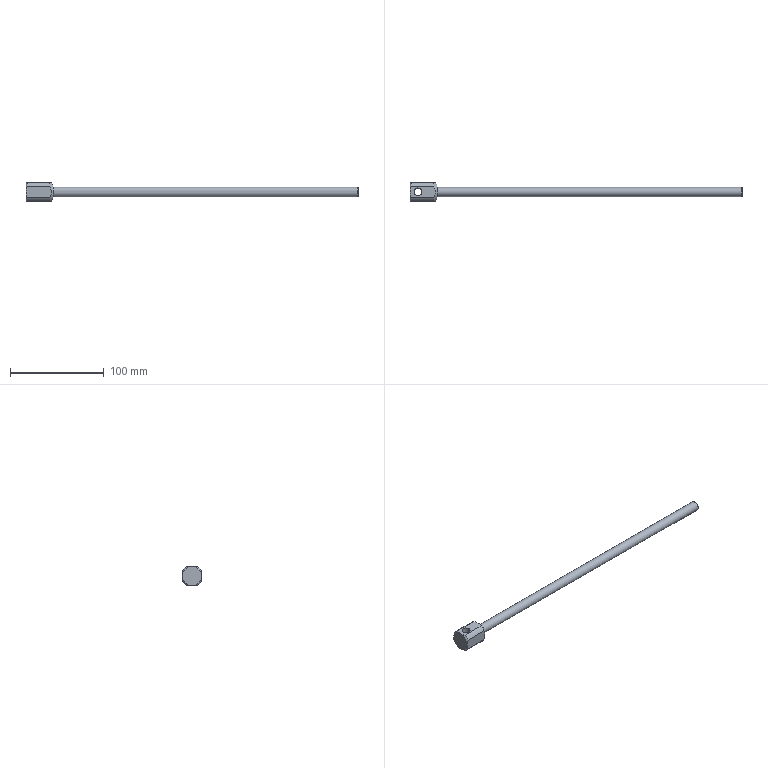Part | STEP file | GAS SHOCK 608S | 1 solid | 20 faces | box 353.5 x 20 x 20 mm | volume 34694 mm3 | plane 7 | cylinder 6 | cone 5 | torus 2 | commonest cylinder face diameters 23 x4 8.5 x1 10 x1
STEP:
#1=CARTESIAN_POINT('',(-27.,-10.,-5.679));
#2=VERTEX_POINT('',#1);
#3=CARTESIAN_POINT('',(-27.,-5.679,-10.));
#4=VERTEX_POINT('',#3);
#5=CARTESIAN_POINT('',(-27.,0.,0.));
#6=DIRECTION('',(1.,0.,0.));
#7=DIRECTION('',(0.,0.,1.));
#8=AXIS2_PLACEMENT_3D('',#5,#6,#7);
#9=CIRCLE('',#8,11.5);
#10=EDGE_CURVE('',#2,#4,#9,.T.);
#11=ORIENTED_EDGE('',*,*,#10,.T.);
#12=CARTESIAN_POINT('',(-3.,-5.679,-10.));
#13=VERTEX_POINT('',#12);
#14=CARTESIAN_POINT('',(-28.5,-5.679,-10.));
#15=DIRECTION('',(1.,0.,0.));
#16=VECTOR('',#15,1000.);
#17=LINE('',#14,#16);
#18=EDGE_CURVE('',#4,#13,#17,.T.);
#19=ORIENTED_EDGE('',*,*,#18,.T.);
#20=CARTESIAN_POINT('',(-3.,-10.,-5.679));
#21=VERTEX_POINT('',#20);
#22=CARTESIAN_POINT('',(-3.,0.,0.));
#23=DIRECTION('',(-1.,0.,0.));
#24=DIRECTION('',(0.,0.,1.));
#25=AXIS2_PLACEMENT_3D('',#22,#23,#24);
#26=CIRCLE('',#25,11.5);
#27=EDGE_CURVE('',#13,#21,#26,.T.);
#28=ORIENTED_EDGE('',*,*,#27,.T.);
#29=CARTESIAN_POINT('',(-28.5,-10.,-5.679));
#30=DIRECTION('',(-1.,0.,0.));
#31=VECTOR('',#30,1000.);
#32=LINE('',#29,#31);
#33=EDGE_CURVE('',#21,#2,#32,.T.);
#34=ORIENTED_EDGE('',*,*,#33,.T.);
#35=EDGE_LOOP('',(#11,#19,#28,#34));
#36=FACE_OUTER_BOUND('',#35,.T.);
#37=CARTESIAN_POINT('',(-28.5,0.,0.));
#38=DIRECTION('',(1.,0.,0.));
#39=DIRECTION('',(0.,0.,-1.));
#40=AXIS2_PLACEMENT_3D('',#37,#38,#39);
#41=CYLINDRICAL_SURFACE('',#40,11.5);
#42=ADVANCED_FACE('',(#36),#41,.T.);
#43=CARTESIAN_POINT('',(-28.5,0.,-10.));
#44=VERTEX_POINT('',#43);
#45=CARTESIAN_POINT('',(-27.,-5.679,-10.));
#46=CARTESIAN_POINT('',(-27.44,-4.788,-10.));
#47=CARTESIAN_POINT('',(-27.813,-3.877,-10.));
#48=CARTESIAN_POINT('',(-28.211,-2.462,-10.));
#49=CARTESIAN_POINT('',(-28.317,-1.982,-10.));
#50=CARTESIAN_POINT('',(-28.462,-1.001,-10.));
#51=CARTESIAN_POINT('',(-28.5,-0.4969,-10.));
#52=CARTESIAN_POINT('',(-28.5,0.,-10.));
#53=B_SPLINE_CURVE_WITH_KNOTS('',3,(#45,#46,#47,#48,#49,#50,#51,#52),.UNSPECIFIED.,.F.,.F.,(4,2,2,4),(0.01277,0.01572,0.01719,0.01867),.UNSPECIFIED.);
#54=EDGE_CURVE('',#4,#44,#53,.T.);
#55=ORIENTED_EDGE('',*,*,#54,.F.);
#56=ORIENTED_EDGE('',*,*,#10,.F.);
#57=CARTESIAN_POINT('',(-28.5,-10.,0.));
#58=VERTEX_POINT('',#57);
#59=CARTESIAN_POINT('',(-28.5,-10.,0.));
#60=CARTESIAN_POINT('',(-28.5,-10.,-0.2479));
#61=CARTESIAN_POINT('',(-28.491,-10.,-0.4984));
#62=CARTESIAN_POINT('',(-28.454,-10.,-0.996));
#63=CARTESIAN_POINT('',(-28.426,-10.,-1.242));
#64=CARTESIAN_POINT('',(-28.318,-10.,-1.975));
#65=CARTESIAN_POINT('',(-28.213,-10.,-2.454));
#66=CARTESIAN_POINT('',(-27.948,-10.,-3.398));
#67=CARTESIAN_POINT('',(-27.788,-10.,-3.863));
#68=CARTESIAN_POINT('',(-27.424,-10.,-4.781));
#69=CARTESIAN_POINT('',(-27.219,-10.,-5.235));
#70=CARTESIAN_POINT('',(-27.,-10.,-5.679));
#71=B_SPLINE_CURVE_WITH_KNOTS('',3,(#59,#60,#61,#62,#63,#64,#65,#66,#67,#68,#69,#70),.UNSPECIFIED.,.F.,.F.,(4,2,2,2,2,4),(0.01208,0.01282,0.01355,0.01502,0.01649,0.01796),.UNSPECIFIED.);
#72=EDGE_CURVE('',#58,#2,#71,.T.);
#73=ORIENTED_EDGE('',*,*,#72,.F.);
#74=CARTESIAN_POINT('',(-28.5,0.,0.));
#75=DIRECTION('',(-1.,0.,0.));
#76=DIRECTION('',(0.,0.,1.));
#77=AXIS2_PLACEMENT_3D('',#74,#75,#76);
#78=CIRCLE('',#77,10.);
#79=EDGE_CURVE('',#44,#58,#78,.T.);
#80=ORIENTED_EDGE('',*,*,#79,.F.);
#81=EDGE_LOOP('',(#55,#56,#73,#80));
#82=FACE_OUTER_BOUND('',#81,.T.);
#83=CARTESIAN_POINT('',(-28.5,0.,0.));
#84=DIRECTION('',(1.,0.,0.));
#85=DIRECTION('',(0.,0.,-1.));
#86=AXIS2_PLACEMENT_3D('',#83,#84,#85);
#87=CONICAL_SURFACE('',#86,10.,0.7854);
#88=ADVANCED_FACE('',(#82),#87,.T.);
#89=CARTESIAN_POINT('',(-27.,-5.679,10.));
#90=VERTEX_POINT('',#89);
#91=CARTESIAN_POINT('',(-27.,-10.,5.679));
#92=VERTEX_POINT('',#91);
#93=CARTESIAN_POINT('',(-27.,0.,0.));
#94=DIRECTION('',(1.,0.,0.));
#95=DIRECTION('',(0.,0.,1.));
#96=AXIS2_PLACEMENT_3D('',#93,#94,#95);
#97=CIRCLE('',#96,11.5);
#98=EDGE_CURVE('',#90,#92,#97,.T.);
#99=ORIENTED_EDGE('',*,*,#98,.T.);
#100=CARTESIAN_POINT('',(-3.,-10.,5.679));
#101=VERTEX_POINT('',#100);
#102=CARTESIAN_POINT('',(-28.5,-10.,5.679));
#103=DIRECTION('',(1.,0.,0.));
#104=VECTOR('',#103,1000.);
#105=LINE('',#102,#104);
#106=EDGE_CURVE('',#92,#101,#105,.T.);
#107=ORIENTED_EDGE('',*,*,#106,.T.);
#108=CARTESIAN_POINT('',(-3.,-5.679,10.));
#109=VERTEX_POINT('',#108);
#110=CARTESIAN_POINT('',(-3.,0.,0.));
#111=DIRECTION('',(-1.,0.,0.));
#112=DIRECTION('',(0.,0.,1.));
#113=AXIS2_PLACEMENT_3D('',#110,#111,#112);
#114=CIRCLE('',#113,11.5);
#115=EDGE_CURVE('',#101,#109,#114,.T.);
#116=ORIENTED_EDGE('',*,*,#115,.T.);
#117=CARTESIAN_POINT('',(-28.5,-5.679,10.));
#118=DIRECTION('',(-1.,0.,0.));
#119=VECTOR('',#118,1000.);
#120=LINE('',#117,#119);
#121=EDGE_CURVE('',#109,#90,#120,.T.);
#122=ORIENTED_EDGE('',*,*,#121,.T.);
#123=EDGE_LOOP('',(#99,#107,#116,#122));
#124=FACE_OUTER_BOUND('',#123,.T.);
#125=CARTESIAN_POINT('',(-28.5,0.,0.));
#126=DIRECTION('',(1.,0.,0.));
#127=DIRECTION('',(0.,0.,-1.));
#128=AXIS2_PLACEMENT_3D('',#125,#126,#127);
#129=CYLINDRICAL_SURFACE('',#128,11.5);
#130=ADVANCED_FACE('',(#124),#129,.T.);
#131=CARTESIAN_POINT('',(-27.,-10.,5.679));
#132=CARTESIAN_POINT('',(-27.218,-10.,5.238));
#133=CARTESIAN_POINT('',(-27.421,-10.,4.789));
#134=CARTESIAN_POINT('',(-27.787,-10.,3.867));
#135=CARTESIAN_POINT('',(-27.95,-10.,3.392));
#136=CARTESIAN_POINT('',(-28.35,-10.,1.964));
#137=CARTESIAN_POINT('',(-28.5,-10.,0.9934));
#138=CARTESIAN_POINT('',(-28.5,-10.,0.));
#139=B_SPLINE_CURVE_WITH_KNOTS('',3,(#131,#132,#133,#134,#135,#136,#137,#138),.UNSPECIFIED.,.F.,.F.,(4,2,2,4),(0.006195,0.007667,0.00914,0.01208),.UNSPECIFIED.);
#140=EDGE_CURVE('',#92,#58,#139,.T.);
#141=ORIENTED_EDGE('',*,*,#140,.F.);
#142=ORIENTED_EDGE('',*,*,#98,.F.);
#143=CARTESIAN_POINT('',(-28.5,0.,10.));
#144=VERTEX_POINT('',#143);
#145=CARTESIAN_POINT('',(-28.5,0.,10.));
#146=CARTESIAN_POINT('',(-28.5,-0.2479,10.));
#147=CARTESIAN_POINT('',(-28.491,-0.4984,10.));
#148=CARTESIAN_POINT('',(-28.454,-0.996,10.));
#149=CARTESIAN_POINT('',(-28.426,-1.242,10.));
#150=CARTESIAN_POINT('',(-28.318,-1.975,10.));
#151=CARTESIAN_POINT('',(-28.213,-2.454,10.));
#152=CARTESIAN_POINT('',(-27.948,-3.398,10.));
#153=CARTESIAN_POINT('',(-27.788,-3.863,10.));
#154=CARTESIAN_POINT('',(-27.424,-4.781,10.));
#155=CARTESIAN_POINT('',(-27.219,-5.235,10.));
#156=CARTESIAN_POINT('',(-27.,-5.679,10.));
#157=B_SPLINE_CURVE_WITH_KNOTS('',3,(#145,#146,#147,#148,#149,#150,#151,#152,#153,#154,#155,#156),.UNSPECIFIED.,.F.,.F.,(4,2,2,2,2,4),(0.01208,0.01282,0.01355,0.01502,0.01649,0.01796),.UNSPECIFIED.);
#158=EDGE_CURVE('',#144,#90,#157,.T.);
#159=ORIENTED_EDGE('',*,*,#158,.F.);
#160=CARTESIAN_POINT('',(-28.5,0.,0.));
#161=DIRECTION('',(-1.,0.,0.));
#162=DIRECTION('',(0.,0.,1.));
#163=AXIS2_PLACEMENT_3D('',#160,#161,#162);
#164=CIRCLE('',#163,10.);
#165=EDGE_CURVE('',#58,#144,#164,.T.);
#166=ORIENTED_EDGE('',*,*,#165,.F.);
#167=EDGE_LOOP('',(#141,#142,#159,#166));
#168=FACE_OUTER_BOUND('',#167,.T.);
#169=CARTESIAN_POINT('',(-28.5,0.,0.));
#170=DIRECTION('',(1.,0.,0.));
#171=DIRECTION('',(0.,0.,-1.));
#172=AXIS2_PLACEMENT_3D('',#169,#170,#171);
#173=CONICAL_SURFACE('',#172,10.,0.7854);
#174=ADVANCED_FACE('',(#168),#173,.T.);
#175=CARTESIAN_POINT('',(-27.,10.,5.679));
#176=VERTEX_POINT('',#175);
#177=CARTESIAN_POINT('',(-27.,5.679,10.));
#178=VERTEX_POINT('',#177);
#179=CARTESIAN_POINT('',(-27.,0.,0.));
#180=DIRECTION('',(1.,0.,0.));
#181=DIRECTION('',(0.,0.,1.));
#182=AXIS2_PLACEMENT_3D('',#179,#180,#181);
#183=CIRCLE('',#182,11.5);
#184=EDGE_CURVE('',#176,#178,#183,.T.);
#185=ORIENTED_EDGE('',*,*,#184,.T.);
#186=CARTESIAN_POINT('',(-3.,5.679,10.));
#187=VERTEX_POINT('',#186);
#188=CARTESIAN_POINT('',(-28.5,5.679,10.));
#189=DIRECTION('',(1.,0.,0.));
#190=VECTOR('',#189,1000.);
#191=LINE('',#188,#190);
#192=EDGE_CURVE('',#178,#187,#191,.T.);
#193=ORIENTED_EDGE('',*,*,#192,.T.);
#194=CARTESIAN_POINT('',(-3.,10.,5.679));
#195=VERTEX_POINT('',#194);
#196=CARTESIAN_POINT('',(-3.,0.,0.));
#197=DIRECTION('',(-1.,0.,0.));
#198=DIRECTION('',(0.,0.,1.));
#199=AXIS2_PLACEMENT_3D('',#196,#197,#198);
#200=CIRCLE('',#199,11.5);
#201=EDGE_CURVE('',#187,#195,#200,.T.);
#202=ORIENTED_EDGE('',*,*,#201,.T.);
#203=CARTESIAN_POINT('',(-28.5,10.,5.679));
#204=DIRECTION('',(-1.,0.,0.));
#205=VECTOR('',#204,1000.);
#206=LINE('',#203,#205);
#207=EDGE_CURVE('',#195,#176,#206,.T.);
#208=ORIENTED_EDGE('',*,*,#207,.T.);
#209=EDGE_LOOP('',(#185,#193,#202,#208));
#210=FACE_OUTER_BOUND('',#209,.T.);
#211=CARTESIAN_POINT('',(-28.5,0.,0.));
#212=DIRECTION('',(1.,0.,0.));
#213=DIRECTION('',(0.,0.,-1.));
#214=AXIS2_PLACEMENT_3D('',#211,#212,#213);
#215=CYLINDRICAL_SURFACE('',#214,11.5);
#216=ADVANCED_FACE('',(#210),#215,.T.);
#217=CARTESIAN_POINT('',(-27.,5.679,10.));
#218=CARTESIAN_POINT('',(-27.218,5.238,10.));
#219=CARTESIAN_POINT('',(-27.421,4.789,10.));
#220=CARTESIAN_POINT('',(-27.787,3.867,10.));
#221=CARTESIAN_POINT('',(-27.95,3.392,10.));
#222=CARTESIAN_POINT('',(-28.35,1.964,10.));
#223=CARTESIAN_POINT('',(-28.5,0.9934,10.));
#224=CARTESIAN_POINT('',(-28.5,0.,10.));
#225=B_SPLINE_CURVE_WITH_KNOTS('',3,(#217,#218,#219,#220,#221,#222,#223,#224),.UNSPECIFIED.,.F.,.F.,(4,2,2,4),(0.006195,0.007667,0.00914,0.01208),.UNSPECIFIED.);
#226=EDGE_CURVE('',#178,#144,#225,.T.);
#227=ORIENTED_EDGE('',*,*,#226,.F.);
#228=ORIENTED_EDGE('',*,*,#184,.F.);
#229=CARTESIAN_POINT('',(-28.5,10.,0.));
#230=VERTEX_POINT('',#229);
#231=CARTESIAN_POINT('',(-28.5,10.,0.));
#232=CARTESIAN_POINT('',(-28.5,10.,0.9898));
#233=CARTESIAN_POINT('',(-28.351,10.,1.963));
#234=CARTESIAN_POINT('',(-27.812,10.,3.883));
#235=CARTESIAN_POINT('',(-27.436,10.,4.796));
#236=CARTESIAN_POINT('',(-27.,10.,5.679));
#237=B_SPLINE_CURVE_WITH_KNOTS('',3,(#231,#232,#233,#234,#235,#236),.UNSPECIFIED.,.F.,.F.,(4,2,4),(0.01867,0.0216,0.02454),.UNSPECIFIED.);
#238=EDGE_CURVE('',#230,#176,#237,.T.);
#239=ORIENTED_EDGE('',*,*,#238,.F.);
#240=CARTESIAN_POINT('',(-28.5,0.,0.));
#241=DIRECTION('',(-1.,0.,0.));
#242=DIRECTION('',(0.,0.,1.));
#243=AXIS2_PLACEMENT_3D('',#240,#241,#242);
#244=CIRCLE('',#243,10.);
#245=EDGE_CURVE('',#144,#230,#244,.T.);
#246=ORIENTED_EDGE('',*,*,#245,.F.);
#247=EDGE_LOOP('',(#227,#228,#239,#246));
#248=FACE_OUTER_BOUND('',#247,.T.);
#249=CARTESIAN_POINT('',(-28.5,0.,0.));
#250=DIRECTION('',(1.,0.,0.));
#251=DIRECTION('',(0.,0.,-1.));
#252=AXIS2_PLACEMENT_3D('',#249,#250,#251);
#253=CONICAL_SURFACE('',#252,10.,0.7854);
#254=ADVANCED_FACE('',(#248),#253,.T.);
#255=CARTESIAN_POINT('',(0.5,0.,5.));
#256=VERTEX_POINT('',#255);
#257=CARTESIAN_POINT('',(0.5,0.,0.));
#258=DIRECTION('',(1.,0.,0.));
#259=DIRECTION('',(0.,0.,1.));
#260=AXIS2_PLACEMENT_3D('',#257,#258,#259);
#261=CIRCLE('',#260,5.);
#262=EDGE_CURVE('',#256,#256,#261,.T.);
#263=ORIENTED_EDGE('',*,*,#262,.T.);
#264=EDGE_LOOP('',(#263));
#265=FACE_OUTER_BOUND('',#264,.T.);
#266=CARTESIAN_POINT('',(324.5,0.,-5.));
#267=VERTEX_POINT('',#266);
#268=CARTESIAN_POINT('',(324.5,0.,0.));
#269=DIRECTION('',(-1.,0.,0.));
#270=DIRECTION('',(0.,0.,-1.));
#271=AXIS2_PLACEMENT_3D('',#268,#269,#270);
#272=CIRCLE('',#271,5.);
#273=EDGE_CURVE('',#267,#267,#272,.T.);
#274=ORIENTED_EDGE('',*,*,#273,.T.);
#275=EDGE_LOOP('',(#274));
#276=FACE_OUTER_BOUND('',#275,.T.);
#277=CARTESIAN_POINT('',(-47.828,0.,0.));
#278=DIRECTION('',(-1.,0.,0.));
#279=DIRECTION('',(0.,0.,1.));
#280=AXIS2_PLACEMENT_3D('',#277,#278,#279);
#281=CYLINDRICAL_SURFACE('',#280,5.);
#282=ADVANCED_FACE('',(#265,#276),#281,.T.);
#283=CARTESIAN_POINT('',(325.,0.,-4.5));
#284=VERTEX_POINT('',#283);
#285=CARTESIAN_POINT('',(325.,0.,0.));
#286=DIRECTION('',(1.,0.,0.));
#287=DIRECTION('',(0.,0.,-1.));
#288=AXIS2_PLACEMENT_3D('',#285,#286,#287);
#289=CIRCLE('',#288,4.5);
#290=EDGE_CURVE('',#284,#284,#289,.T.);
#291=ORIENTED_EDGE('',*,*,#290,.T.);
#292=EDGE_LOOP('',(#291));
#293=FACE_OUTER_BOUND('',#292,.T.);
#294=CARTESIAN_POINT('',(325.,0.,0.));
#295=DIRECTION('',(1.,0.,0.));
#296=DIRECTION('',(0.,0.,-1.));
#297=AXIS2_PLACEMENT_3D('',#294,#295,#296);
#298=PLANE('',#297);
#299=ADVANCED_FACE('',(#293),#298,.T.);
#300=ORIENTED_EDGE('',*,*,#262,.F.);
#301=EDGE_LOOP('',(#300));
#302=FACE_OUTER_BOUND('',#301,.T.);
#303=CARTESIAN_POINT('',(0.,0.,4.5));
#304=VERTEX_POINT('',#303);
#305=CARTESIAN_POINT('',(0.,0.,0.));
#306=DIRECTION('',(-1.,0.,0.));
#307=DIRECTION('',(0.,0.,1.));
#308=AXIS2_PLACEMENT_3D('',#305,#306,#307);
#309=CIRCLE('',#308,4.5);
#310=EDGE_CURVE('',#304,#304,#309,.T.);
#311=ORIENTED_EDGE('',*,*,#310,.F.);
#312=EDGE_LOOP('',(#311));
#313=FACE_OUTER_BOUND('',#312,.T.);
#314=CARTESIAN_POINT('',(0.5,0.,0.));
#315=DIRECTION('',(-1.,0.,0.));
#316=DIRECTION('',(0.,0.,1.));
#317=AXIS2_PLACEMENT_3D('',#314,#315,#316);
#318=TOROIDAL_SURFACE('',#317,4.5,0.5);
#319=ADVANCED_FACE('',(#302,#313),#318,.T.);
#320=ORIENTED_EDGE('',*,*,#290,.F.);
#321=EDGE_LOOP('',(#320));
#322=FACE_OUTER_BOUND('',#321,.T.);
#323=ORIENTED_EDGE('',*,*,#273,.F.);
#324=EDGE_LOOP('',(#323));
#325=FACE_OUTER_BOUND('',#324,.T.);
#326=CARTESIAN_POINT('',(324.5,0.,0.));
#327=DIRECTION('',(1.,0.,0.));
#328=DIRECTION('',(0.,0.,-1.));
#329=AXIS2_PLACEMENT_3D('',#326,#327,#328);
#330=TOROIDAL_SURFACE('',#329,4.5,0.5);
#331=ADVANCED_FACE('',(#322,#325),#330,.T.);
#332=CARTESIAN_POINT('',(-3.,10.,-5.679));
#333=VERTEX_POINT('',#332);
#334=CARTESIAN_POINT('',(-3.,5.679,-10.));
#335=VERTEX_POINT('',#334);
#336=CARTESIAN_POINT('',(-3.,0.,0.));
#337=DIRECTION('',(-1.,0.,0.));
#338=DIRECTION('',(0.,0.,1.));
#339=AXIS2_PLACEMENT_3D('',#336,#337,#338);
#340=CIRCLE('',#339,11.5);
#341=EDGE_CURVE('',#333,#335,#340,.T.);
#342=ORIENTED_EDGE('',*,*,#341,.T.);
#343=CARTESIAN_POINT('',(-27.,5.679,-10.));
#344=VERTEX_POINT('',#343);
#345=CARTESIAN_POINT('',(-28.5,5.679,-10.));
#346=DIRECTION('',(-1.,0.,0.));
#347=VECTOR('',#346,1000.);
#348=LINE('',#345,#347);
#349=EDGE_CURVE('',#335,#344,#348,.T.);
#350=ORIENTED_EDGE('',*,*,#349,.T.);
#351=CARTESIAN_POINT('',(-27.,10.,-5.679));
#352=VERTEX_POINT('',#351);
#353=CARTESIAN_POINT('',(-27.,0.,0.));
#354=DIRECTION('',(1.,0.,0.));
#355=DIRECTION('',(0.,0.,1.));
#356=AXIS2_PLACEMENT_3D('',#353,#354,#355);
#357=CIRCLE('',#356,11.5);
#358=EDGE_CURVE('',#344,#352,#357,.T.);
#359=ORIENTED_EDGE('',*,*,#358,.T.);
#360=CARTESIAN_POINT('',(-28.5,10.,-5.679));
#361=DIRECTION('',(1.,0.,0.));
#362=VECTOR('',#361,1000.);
#363=LINE('',#360,#362);
#364=EDGE_CURVE('',#352,#333,#363,.T.);
#365=ORIENTED_EDGE('',*,*,#364,.T.);
#366=EDGE_LOOP('',(#342,#350,#359,#365));
#367=FACE_OUTER_BOUND('',#366,.T.);
#368=CARTESIAN_POINT('',(-28.5,0.,0.));
#369=DIRECTION('',(1.,0.,0.));
#370=DIRECTION('',(0.,0.,-1.));
#371=AXIS2_PLACEMENT_3D('',#368,#369,#370);
#372=CYLINDRICAL_SURFACE('',#371,11.5);
#373=ADVANCED_FACE('',(#367),#372,.T.);
#374=CARTESIAN_POINT('',(-28.5,0.,0.));
#375=DIRECTION('',(-1.,0.,0.));
#376=DIRECTION('',(0.,0.,1.));
#377=AXIS2_PLACEMENT_3D('',#374,#375,#376);
#378=CIRCLE('',#377,10.);
#379=EDGE_CURVE('',#230,#44,#378,.T.);
#380=ORIENTED_EDGE('',*,*,#379,.T.);
#381=ORIENTED_EDGE('',*,*,#79,.T.);
#382=ORIENTED_EDGE('',*,*,#165,.T.);
#383=ORIENTED_EDGE('',*,*,#245,.T.);
#384=EDGE_LOOP('',(#380,#381,#382,#383));
#385=FACE_OUTER_BOUND('',#384,.T.);
#386=CARTESIAN_POINT('',(-28.5,0.,0.));
#387=DIRECTION('',(-1.,0.,0.));
#388=DIRECTION('',(0.,0.,1.));
#389=AXIS2_PLACEMENT_3D('',#386,#387,#388);
#390=PLANE('',#389);
#391=ADVANCED_FACE('',(#385),#390,.T.);
#392=CARTESIAN_POINT('',(0.,0.,8.5));
#393=VERTEX_POINT('',#392);
#394=CARTESIAN_POINT('',(0.,0.,0.));
#395=DIRECTION('',(1.,0.,0.));
#396=DIRECTION('',(0.,0.,1.));
#397=AXIS2_PLACEMENT_3D('',#394,#395,#396);
#398=CIRCLE('',#397,8.5);
#399=EDGE_CURVE('',#393,#393,#398,.T.);
#400=ORIENTED_EDGE('',*,*,#399,.T.);
#401=EDGE_LOOP('',(#400));
#402=FACE_OUTER_BOUND('',#401,.T.);
#403=ORIENTED_EDGE('',*,*,#310,.T.);
#404=EDGE_LOOP('',(#403));
#405=FACE_BOUND('',#404,.T.);
#406=CARTESIAN_POINT('',(0.,0.,0.));
#407=DIRECTION('',(-1.,0.,0.));
#408=DIRECTION('',(0.,0.,1.));
#409=AXIS2_PLACEMENT_3D('',#406,#407,#408);
#410=PLANE('',#409);
#411=ADVANCED_FACE('',(#402,#405),#410,.F.);
#412=CARTESIAN_POINT('',(-28.5,0.,-10.));
#413=CARTESIAN_POINT('',(-28.5,0.9898,-10.));
#414=CARTESIAN_POINT('',(-28.351,1.963,-10.));
#415=CARTESIAN_POINT('',(-27.812,3.883,-10.));
#416=CARTESIAN_POINT('',(-27.436,4.796,-10.));
#417=CARTESIAN_POINT('',(-27.,5.679,-10.));
#418=B_SPLINE_CURVE_WITH_KNOTS('',3,(#412,#413,#414,#415,#416,#417),.UNSPECIFIED.,.F.,.F.,(4,2,4),(0.01867,0.0216,0.02454),.UNSPECIFIED.);
#419=EDGE_CURVE('',#44,#344,#418,.T.);
#420=ORIENTED_EDGE('',*,*,#419,.F.);
#421=ORIENTED_EDGE('',*,*,#379,.F.);
#422=CARTESIAN_POINT('',(-27.,10.,-5.679));
#423=CARTESIAN_POINT('',(-27.44,10.,-4.788));
#424=CARTESIAN_POINT('',(-27.813,10.,-3.877));
#425=CARTESIAN_POINT('',(-28.211,10.,-2.462));
#426=CARTESIAN_POINT('',(-28.317,10.,-1.982));
#427=CARTESIAN_POINT('',(-28.462,10.,-1.001));
#428=CARTESIAN_POINT('',(-28.5,10.,-0.4969));
#429=CARTESIAN_POINT('',(-28.5,10.,0.));
#430=B_SPLINE_CURVE_WITH_KNOTS('',3,(#422,#423,#424,#425,#426,#427,#428,#429),.UNSPECIFIED.,.F.,.F.,(4,2,2,4),(0.01277,0.01572,0.01719,0.01867),.UNSPECIFIED.);
#431=EDGE_CURVE('',#352,#230,#430,.T.);
#432=ORIENTED_EDGE('',*,*,#431,.F.);
#433=ORIENTED_EDGE('',*,*,#358,.F.);
#434=EDGE_LOOP('',(#420,#421,#432,#433));
#435=FACE_OUTER_BOUND('',#434,.T.);
#436=CARTESIAN_POINT('',(-28.5,0.,0.));
#437=DIRECTION('',(1.,0.,0.));
#438=DIRECTION('',(0.,0.,-1.));
#439=AXIS2_PLACEMENT_3D('',#436,#437,#438);
#440=CONICAL_SURFACE('',#439,10.,0.7854);
#441=ADVANCED_FACE('',(#435),#440,.T.);
#442=CARTESIAN_POINT('',(-3.,5.679,-10.));
#443=CARTESIAN_POINT('',(-2.782,5.237,-10.));
#444=CARTESIAN_POINT('',(-2.579,4.788,-10.));
#445=CARTESIAN_POINT('',(-2.214,3.87,-10.));
#446=CARTESIAN_POINT('',(-2.052,3.399,-10.));
#447=CARTESIAN_POINT('',(-1.648,1.959,-10.));
#448=CARTESIAN_POINT('',(-1.499,0.9842,-10.));
#449=CARTESIAN_POINT('',(-1.5,-0.5037,-10.));
#450=CARTESIAN_POINT('',(-1.539,-1.006,-10.));
#451=CARTESIAN_POINT('',(-1.683,-1.984,-10.));
#452=CARTESIAN_POINT('',(-1.789,-2.463,-10.));
#453=CARTESIAN_POINT('',(-2.054,-3.405,-10.));
#454=CARTESIAN_POINT('',(-2.214,-3.868,-10.));
#455=CARTESIAN_POINT('',(-2.577,-4.782,-10.));
#456=CARTESIAN_POINT('',(-2.78,-5.234,-10.));
#457=CARTESIAN_POINT('',(-3.,-5.679,-10.));
#458=B_SPLINE_CURVE_WITH_KNOTS('',3,(#442,#443,#444,#445,#446,#447,#448,#449,#450,#451,#452,#453,#454,#455,#456,#457),.UNSPECIFIED.,.F.,.F.,(4,2,2,2,2,2,2,4),(0.03258,0.03405,0.03553,0.03847,0.03995,0.04142,0.04289,0.04437),.UNSPECIFIED.);
#459=EDGE_CURVE('',#335,#13,#458,.T.);
#460=ORIENTED_EDGE('',*,*,#459,.F.);
#461=ORIENTED_EDGE('',*,*,#341,.F.);
#462=CARTESIAN_POINT('',(-3.,10.,5.679));
#463=CARTESIAN_POINT('',(-2.782,10.,5.237));
#464=CARTESIAN_POINT('',(-2.579,10.,4.788));
#465=CARTESIAN_POINT('',(-2.214,10.,3.87));
#466=CARTESIAN_POINT('',(-2.052,10.,3.399));
#467=CARTESIAN_POINT('',(-1.648,10.,1.959));
#468=CARTESIAN_POINT('',(-1.499,10.,0.9842));
#469=CARTESIAN_POINT('',(-1.5,10.,-0.5037));
#470=CARTESIAN_POINT('',(-1.539,10.,-1.006));
#471=CARTESIAN_POINT('',(-1.683,10.,-1.984));
#472=CARTESIAN_POINT('',(-1.789,10.,-2.463));
#473=CARTESIAN_POINT('',(-2.054,10.,-3.405));
#474=CARTESIAN_POINT('',(-2.214,10.,-3.868));
#475=CARTESIAN_POINT('',(-2.577,10.,-4.782));
#476=CARTESIAN_POINT('',(-2.78,10.,-5.234));
#477=CARTESIAN_POINT('',(-3.,10.,-5.679));
#478=B_SPLINE_CURVE_WITH_KNOTS('',3,(#462,#463,#464,#465,#466,#467,#468,#469,#470,#471,#472,#473,#474,#475,#476,#477),.UNSPECIFIED.,.F.,.F.,(4,2,2,2,2,2,2,4),(0.03258,0.03405,0.03553,0.03847,0.03995,0.04142,0.04289,0.04437),.UNSPECIFIED.);
#479=EDGE_CURVE('',#195,#333,#478,.T.);
#480=ORIENTED_EDGE('',*,*,#479,.F.);
#481=ORIENTED_EDGE('',*,*,#201,.F.);
#482=CARTESIAN_POINT('',(-3.,-5.679,10.));
#483=CARTESIAN_POINT('',(-2.781,-5.236,10.));
#484=CARTESIAN_POINT('',(-2.576,-4.781,10.));
#485=CARTESIAN_POINT('',(-2.211,-3.86,10.));
#486=CARTESIAN_POINT('',(-2.051,-3.394,10.));
#487=CARTESIAN_POINT('',(-1.785,-2.449,10.));
#488=CARTESIAN_POINT('',(-1.681,-1.969,10.));
#489=CARTESIAN_POINT('',(-1.573,-1.237,10.));
#490=CARTESIAN_POINT('',(-1.546,-0.9908,10.));
#491=CARTESIAN_POINT('',(-1.509,-0.4941,10.));
#492=CARTESIAN_POINT('',(-1.5,-0.243,10.));
#493=CARTESIAN_POINT('',(-1.501,0.9989,10.));
#494=CARTESIAN_POINT('',(-1.651,1.969,10.));
#495=CARTESIAN_POINT('',(-2.051,3.396,10.));
#496=CARTESIAN_POINT('',(-2.214,3.87,10.));
#497=CARTESIAN_POINT('',(-2.58,4.79,10.));
#498=CARTESIAN_POINT('',(-2.783,5.239,10.));
#499=CARTESIAN_POINT('',(-3.,5.679,10.));
#500=B_SPLINE_CURVE_WITH_KNOTS('',3,(#482,#483,#484,#485,#486,#487,#488,#489,#490,#491,#492,#493,#494,#495,#496,#497,#498,#499),.UNSPECIFIED.,.F.,.F.,(4,2,2,2,2,2,2,2,4),(0.009277,0.01075,0.01222,0.01369,0.01443,0.01516,0.01811,0.01958,0.02105),.UNSPECIFIED.);
#501=EDGE_CURVE('',#109,#187,#500,.T.);
#502=ORIENTED_EDGE('',*,*,#501,.F.);
#503=ORIENTED_EDGE('',*,*,#115,.F.);
#504=CARTESIAN_POINT('',(-3.,-10.,-5.679));
#505=CARTESIAN_POINT('',(-2.781,-10.,-5.236));
#506=CARTESIAN_POINT('',(-2.576,-10.,-4.781));
#507=CARTESIAN_POINT('',(-2.211,-10.,-3.86));
#508=CARTESIAN_POINT('',(-2.051,-10.,-3.394));
#509=CARTESIAN_POINT('',(-1.785,-10.,-2.449));
#510=CARTESIAN_POINT('',(-1.681,-10.,-1.969));
#511=CARTESIAN_POINT('',(-1.573,-10.,-1.237));
#512=CARTESIAN_POINT('',(-1.546,-10.,-0.9908));
#513=CARTESIAN_POINT('',(-1.509,-10.,-0.4941));
#514=CARTESIAN_POINT('',(-1.5,-10.,-0.243));
#515=CARTESIAN_POINT('',(-1.501,-10.,0.9989));
#516=CARTESIAN_POINT('',(-1.651,-10.,1.969));
#517=CARTESIAN_POINT('',(-2.051,-10.,3.396));
#518=CARTESIAN_POINT('',(-2.214,-10.,3.87));
#519=CARTESIAN_POINT('',(-2.58,-10.,4.79));
#520=CARTESIAN_POINT('',(-2.783,-10.,5.239));
#521=CARTESIAN_POINT('',(-3.,-10.,5.679));
#522=B_SPLINE_CURVE_WITH_KNOTS('',3,(#504,#505,#506,#507,#508,#509,#510,#511,#512,#513,#514,#515,#516,#517,#518,#519,#520,#521),.UNSPECIFIED.,.F.,.F.,(4,2,2,2,2,2,2,2,4),(0.009277,0.01075,0.01222,0.01369,0.01443,0.01516,0.01811,0.01958,0.02105),.UNSPECIFIED.);
#523=EDGE_CURVE('',#21,#101,#522,.T.);
#524=ORIENTED_EDGE('',*,*,#523,.F.);
#525=ORIENTED_EDGE('',*,*,#27,.F.);
#526=EDGE_LOOP('',(#460,#461,#480,#481,#502,#503,#524,#525));
#527=FACE_OUTER_BOUND('',#526,.T.);
#528=ORIENTED_EDGE('',*,*,#399,.F.);
#529=EDGE_LOOP('',(#528));
#530=FACE_BOUND('',#529,.T.);
#531=CARTESIAN_POINT('',(-3.,0.,0.));
#532=DIRECTION('',(-1.,0.,0.));
#533=DIRECTION('',(0.,0.,1.));
#534=AXIS2_PLACEMENT_3D('',#531,#532,#533);
#535=CONICAL_SURFACE('',#534,11.5,0.7854);
#536=ADVANCED_FACE('',(#527,#530),#535,.T.);
#537=ORIENTED_EDGE('',*,*,#431,.T.);
#538=ORIENTED_EDGE('',*,*,#238,.T.);
#539=ORIENTED_EDGE('',*,*,#207,.F.);
#540=ORIENTED_EDGE('',*,*,#479,.T.);
#541=ORIENTED_EDGE('',*,*,#364,.F.);
#542=EDGE_LOOP('',(#537,#538,#539,#540,#541));
#543=FACE_OUTER_BOUND('',#542,.T.);
#544=CARTESIAN_POINT('',(0.,10.,-8.195));
#545=DIRECTION('',(0.,-1.,0.));
#546=DIRECTION('',(0.,0.,-1.));
#547=AXIS2_PLACEMENT_3D('',#544,#545,#546);
#548=PLANE('',#547);
#549=ADVANCED_FACE('',(#543),#548,.F.);
#550=CARTESIAN_POINT('',(-20.,4.25,10.));
#551=VERTEX_POINT('',#550);
#552=CARTESIAN_POINT('',(-20.,0.,10.));
#553=DIRECTION('',(0.,0.,-1.));
#554=DIRECTION('',(0.,1.,0.));
#555=AXIS2_PLACEMENT_3D('',#552,#553,#554);
#556=CIRCLE('',#555,4.25);
#557=EDGE_CURVE('',#551,#551,#556,.T.);
#558=ORIENTED_EDGE('',*,*,#557,.T.);
#559=EDGE_LOOP('',(#558));
#560=FACE_BOUND('',#559,.T.);
#561=ORIENTED_EDGE('',*,*,#226,.T.);
#562=ORIENTED_EDGE('',*,*,#158,.T.);
#563=ORIENTED_EDGE('',*,*,#121,.F.);
#564=ORIENTED_EDGE('',*,*,#501,.T.);
#565=ORIENTED_EDGE('',*,*,#192,.F.);
#566=EDGE_LOOP('',(#561,#562,#563,#564,#565));
#567=FACE_OUTER_BOUND('',#566,.T.);
#568=CARTESIAN_POINT('',(0.,8.195,10.));
#569=DIRECTION('',(0.,0.,-1.));
#570=DIRECTION('',(0.,1.,0.));
#571=AXIS2_PLACEMENT_3D('',#568,#569,#570);
#572=PLANE('',#571);
#573=ADVANCED_FACE('',(#560,#567),#572,.F.);
#574=ORIENTED_EDGE('',*,*,#140,.T.);
#575=ORIENTED_EDGE('',*,*,#72,.T.);
#576=ORIENTED_EDGE('',*,*,#33,.F.);
#577=ORIENTED_EDGE('',*,*,#523,.T.);
#578=ORIENTED_EDGE('',*,*,#106,.F.);
#579=EDGE_LOOP('',(#574,#575,#576,#577,#578));
#580=FACE_OUTER_BOUND('',#579,.T.);
#581=CARTESIAN_POINT('',(0.,-10.,8.195));
#582=DIRECTION('',(0.,1.,0.));
#583=DIRECTION('',(0.,0.,1.));
#584=AXIS2_PLACEMENT_3D('',#581,#582,#583);
#585=PLANE('',#584);
#586=ADVANCED_FACE('',(#580),#585,.F.);
#587=CARTESIAN_POINT('',(-20.,-4.25,-10.));
#588=VERTEX_POINT('',#587);
#589=CARTESIAN_POINT('',(-20.,0.,-10.));
#590=DIRECTION('',(0.,0.,1.));
#591=DIRECTION('',(0.,-1.,0.));
#592=AXIS2_PLACEMENT_3D('',#589,#590,#591);
#593=CIRCLE('',#592,4.25);
#594=EDGE_CURVE('',#588,#588,#593,.T.);
#595=ORIENTED_EDGE('',*,*,#594,.T.);
#596=EDGE_LOOP('',(#595));
#597=FACE_BOUND('',#596,.T.);
#598=ORIENTED_EDGE('',*,*,#54,.T.);
#599=ORIENTED_EDGE('',*,*,#419,.T.);
#600=ORIENTED_EDGE('',*,*,#349,.F.);
#601=ORIENTED_EDGE('',*,*,#459,.T.);
#602=ORIENTED_EDGE('',*,*,#18,.F.);
#603=EDGE_LOOP('',(#598,#599,#600,#601,#602));
#604=FACE_OUTER_BOUND('',#603,.T.);
#605=CARTESIAN_POINT('',(0.,-8.195,-10.));
#606=DIRECTION('',(0.,0.,1.));
#607=DIRECTION('',(0.,-1.,0.));
#608=AXIS2_PLACEMENT_3D('',#605,#606,#607);
#609=PLANE('',#608);
#610=ADVANCED_FACE('',(#597,#604),#609,.F.);
#611=ORIENTED_EDGE('',*,*,#594,.F.);
#612=EDGE_LOOP('',(#611));
#613=FACE_OUTER_BOUND('',#612,.T.);
#614=ORIENTED_EDGE('',*,*,#557,.F.);
#615=EDGE_LOOP('',(#614));
#616=FACE_OUTER_BOUND('',#615,.T.);
#617=CARTESIAN_POINT('',(-20.,0.,-14.25));
#618=DIRECTION('',(0.,0.,1.));
#619=DIRECTION('',(1.,0.,0.));
#620=AXIS2_PLACEMENT_3D('',#617,#618,#619);
#621=CYLINDRICAL_SURFACE('',#620,4.25);
#622=ADVANCED_FACE('',(#613,#616),#621,.F.);
#623=CLOSED_SHELL('',(#42,#88,#130,#174,#216,#254,#282,#299,#319,#331,#373,#391,#411,#441,#536,#549,#573,#586,#610,#622));
#624=MANIFOLD_SOLID_BREP('',#623);
#625=CARTESIAN_POINT('',(0.,0.,0.));
#626=DIRECTION('',(0.,0.,1.));
#627=DIRECTION('',(1.,0.,0.));
#628=AXIS2_PLACEMENT_3D('',#625,#626,#627);
#629=(LENGTH_UNIT()NAMED_UNIT(*)SI_UNIT(.MILLI.,.METRE.));
#630=UNCERTAINTY_MEASURE_WITH_UNIT(LENGTH_MEASURE(0.00001),#629,'','');
#631=(NAMED_UNIT(*)PLANE_ANGLE_UNIT()SI_UNIT($,.RADIAN.));
#632=(NAMED_UNIT(*)SI_UNIT($,.STERADIAN.)SOLID_ANGLE_UNIT());
#633=(GEOMETRIC_REPRESENTATION_CONTEXT(3)GLOBAL_UNCERTAINTY_ASSIGNED_CONTEXT((#630))GLOBAL_UNIT_ASSIGNED_CONTEXT((#629,#631,#632))REPRESENTATION_CONTEXT('',''));
#634=ADVANCED_BREP_SHAPE_REPRESENTATION('',(#624,#628),#633);